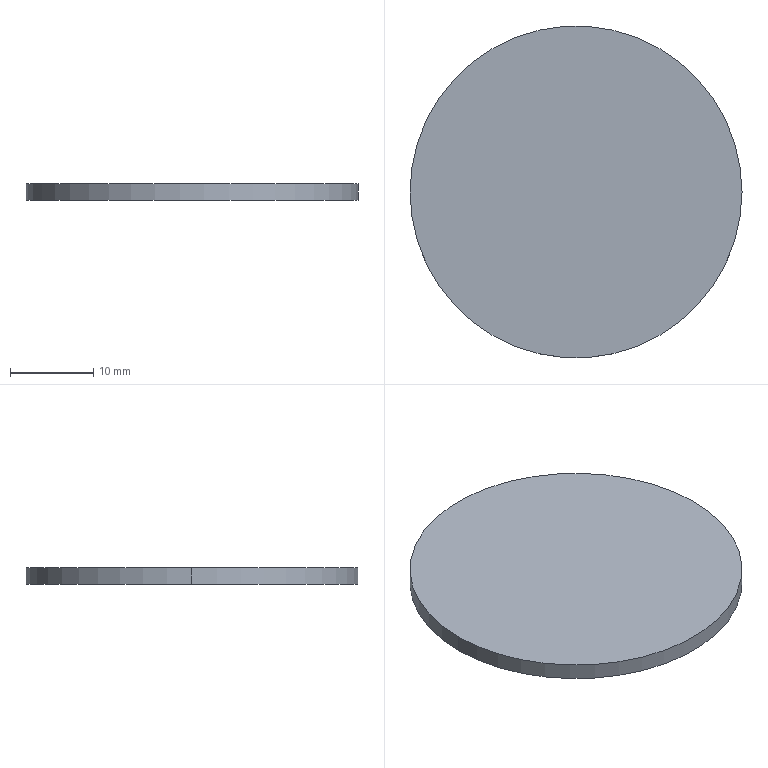Part | SolidWorks | features FlatPattern 1, SMBaseFlange 1, SheetMetal 1 | 1 solid | 4 faces | box 40 x 40 x 2 mm | volume 2513 mm3 | cylinder 2 | plane 2 | commonest cylinder face diameters 40 x2
STEP:
#1=CARTESIAN_POINT('',(20.,0.,-2.));
#2=VERTEX_POINT('',#1);
#3=CARTESIAN_POINT('',(-20.,0.,-2.));
#4=VERTEX_POINT('',#3);
#5=CARTESIAN_POINT('',(0.,0.,-2.));
#6=DIRECTION('',(0.,0.,1.));
#7=DIRECTION('',(1.,0.,0.));
#8=AXIS2_PLACEMENT_3D('',#5,#6,#7);
#9=CIRCLE('',#8,20.);
#10=EDGE_CURVE('',#2,#4,#9,.T.);
#11=ORIENTED_EDGE('',*,*,#10,.T.);
#12=CARTESIAN_POINT('',(-20.,0.,0.));
#13=VERTEX_POINT('',#12);
#14=CARTESIAN_POINT('',(-20.,0.,-2.));
#15=DIRECTION('',(0.,0.,1.));
#16=VECTOR('',#15,1000.);
#17=LINE('',#14,#16);
#18=EDGE_CURVE('',#4,#13,#17,.T.);
#19=ORIENTED_EDGE('',*,*,#18,.T.);
#20=CARTESIAN_POINT('',(20.,0.,0.));
#21=VERTEX_POINT('',#20);
#22=CARTESIAN_POINT('',(0.,0.,0.));
#23=DIRECTION('',(0.,0.,1.));
#24=DIRECTION('',(1.,0.,0.));
#25=AXIS2_PLACEMENT_3D('',#22,#23,#24);
#26=CIRCLE('',#25,20.);
#27=EDGE_CURVE('',#21,#13,#26,.T.);
#28=ORIENTED_EDGE('',*,*,#27,.F.);
#29=CARTESIAN_POINT('',(20.,0.,-2.));
#30=DIRECTION('',(0.,0.,1.));
#31=VECTOR('',#30,1000.);
#32=LINE('',#29,#31);
#33=EDGE_CURVE('',#2,#21,#32,.T.);
#34=ORIENTED_EDGE('',*,*,#33,.F.);
#35=EDGE_LOOP('',(#11,#19,#28,#34));
#36=FACE_OUTER_BOUND('',#35,.T.);
#37=CARTESIAN_POINT('',(0.,0.,-2.));
#38=DIRECTION('',(0.,0.,1.));
#39=DIRECTION('',(1.,0.,0.));
#40=AXIS2_PLACEMENT_3D('',#37,#38,#39);
#41=CYLINDRICAL_SURFACE('',#40,20.);
#42=ADVANCED_FACE('',(#36),#41,.T.);
#43=ORIENTED_EDGE('',*,*,#18,.F.);
#44=CARTESIAN_POINT('',(0.,0.,-2.));
#45=DIRECTION('',(0.,0.,1.));
#46=DIRECTION('',(1.,0.,0.));
#47=AXIS2_PLACEMENT_3D('',#44,#45,#46);
#48=CIRCLE('',#47,20.);
#49=EDGE_CURVE('',#4,#2,#48,.T.);
#50=ORIENTED_EDGE('',*,*,#49,.T.);
#51=ORIENTED_EDGE('',*,*,#33,.T.);
#52=CARTESIAN_POINT('',(0.,0.,0.));
#53=DIRECTION('',(0.,0.,1.));
#54=DIRECTION('',(1.,0.,0.));
#55=AXIS2_PLACEMENT_3D('',#52,#53,#54);
#56=CIRCLE('',#55,20.);
#57=EDGE_CURVE('',#13,#21,#56,.T.);
#58=ORIENTED_EDGE('',*,*,#57,.F.);
#59=EDGE_LOOP('',(#43,#50,#51,#58));
#60=FACE_OUTER_BOUND('',#59,.T.);
#61=CARTESIAN_POINT('',(0.,0.,-2.));
#62=DIRECTION('',(0.,0.,1.));
#63=DIRECTION('',(1.,0.,0.));
#64=AXIS2_PLACEMENT_3D('',#61,#62,#63);
#65=CYLINDRICAL_SURFACE('',#64,20.);
#66=ADVANCED_FACE('',(#60),#65,.T.);
#67=ORIENTED_EDGE('',*,*,#10,.F.);
#68=ORIENTED_EDGE('',*,*,#49,.F.);
#69=EDGE_LOOP('',(#67,#68));
#70=FACE_OUTER_BOUND('',#69,.T.);
#71=CARTESIAN_POINT('',(0.,0.,-2.));
#72=DIRECTION('',(0.,0.,1.));
#73=DIRECTION('',(1.,0.,0.));
#74=AXIS2_PLACEMENT_3D('',#71,#72,#73);
#75=PLANE('',#74);
#76=ADVANCED_FACE('',(#70),#75,.F.);
#77=ORIENTED_EDGE('',*,*,#27,.T.);
#78=ORIENTED_EDGE('',*,*,#57,.T.);
#79=EDGE_LOOP('',(#77,#78));
#80=FACE_OUTER_BOUND('',#79,.T.);
#81=CARTESIAN_POINT('',(0.,0.,0.));
#82=DIRECTION('',(0.,0.,1.));
#83=DIRECTION('',(1.,0.,0.));
#84=AXIS2_PLACEMENT_3D('',#81,#82,#83);
#85=PLANE('',#84);
#86=ADVANCED_FACE('',(#80),#85,.T.);
#87=CLOSED_SHELL('',(#42,#66,#76,#86));
#88=MANIFOLD_SOLID_BREP('',#87);
#89=CARTESIAN_POINT('',(0.,0.,0.));
#90=DIRECTION('',(0.,0.,1.));
#91=DIRECTION('',(1.,0.,0.));
#92=AXIS2_PLACEMENT_3D('',#89,#90,#91);
#93=(LENGTH_UNIT()NAMED_UNIT(*)SI_UNIT(.MILLI.,.METRE.));
#94=UNCERTAINTY_MEASURE_WITH_UNIT(LENGTH_MEASURE(0.00001),#93,'','');
#95=(NAMED_UNIT(*)PLANE_ANGLE_UNIT()SI_UNIT($,.RADIAN.));
#96=(NAMED_UNIT(*)SI_UNIT($,.STERADIAN.)SOLID_ANGLE_UNIT());
#97=(GEOMETRIC_REPRESENTATION_CONTEXT(3)GLOBAL_UNCERTAINTY_ASSIGNED_CONTEXT((#94))GLOBAL_UNIT_ASSIGNED_CONTEXT((#93,#95,#96))REPRESENTATION_CONTEXT('',''));
#98=ADVANCED_BREP_SHAPE_REPRESENTATION('',(#88,#92),#97);